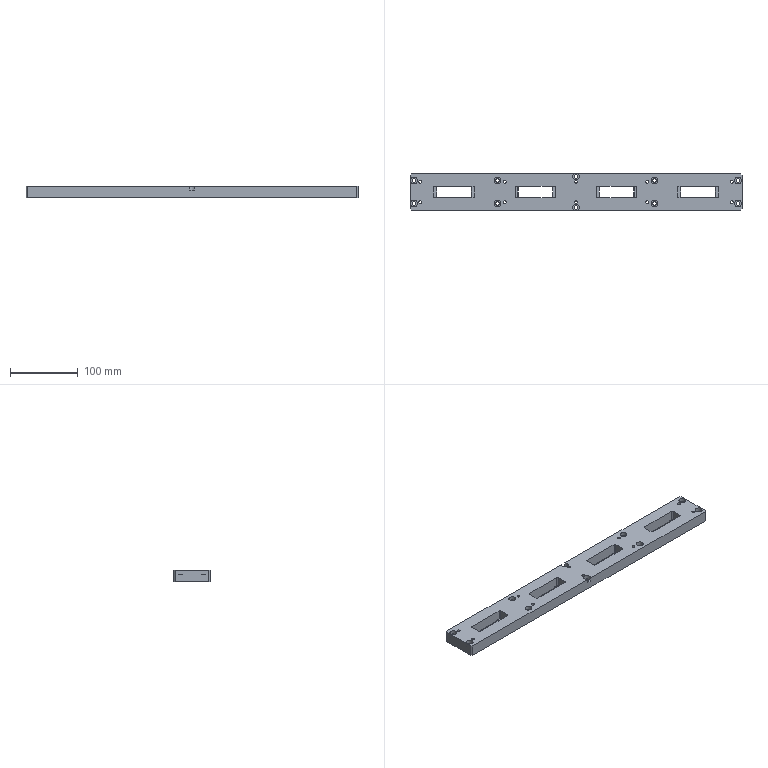NC program | NX | posted with a generic post | part box 490 x 54 x 17 mm
Lines 8259 to 8955 of 8955:
(ZLEVEL_PROFILE_2 , TOOL : D4R0.5)
N16468 T05 M6
N16470 G54
N16472 G17 G0 G90 X448.389 Y-32.658 S8500 M3
N16474 G43 Z30. H5
N16476 Z-13.1
N16478 G94 G1 Z-14.6 F2500.
N16480 X448.817 Y-33.4
N16482 G3 X449.164 Y-33.6 R0.4
N16484 G1 X449.175 Y-33.595
N16486 X449.187 Y-33.303
N16488 X449.191 Y-31.902
N16490 X449.189 Y-20.697
N16492 X449.179 Y-20.401
N16494 X449.164 Y-20.4
N16496 X449.093 Z-14.7
N16498 Y-33.6
N16500 X448.993 Z-14.8
N16502 Y-20.4
N16504 X448.893 Z-14.9
N16506 Y-33.6
N16508 X448.793 Z-15.
N16510 Y-20.4
N16512 X448.693 Z-15.1
N16514 Y-33.6
N16516 X448.575 Z-15.2
N16518 X448.588 Y-33.303
N16520 X448.591 Y-22.098
N16522 X448.579 Y-20.417
N16524 X448.577 Y-20.401
N16526 X448.552 Y-20.4
N16528 X448.163 Z-15.3
N16530 G2 X448.473 Y-20.487 R0.521
N16532 G1 X448.489 Y-22.098
N16534 X448.49 Y-32.182
N16536 X448.471 Y-33.537
N16538 X448.413 Y-33.562
N16540 X448.103 Y-33.6
N16542 X448.15 Y-33.54 Z-15.35
N16544 X448.198 Y-33.482 Z-15.4
N16546 X448.299 Y-33.481
N16548 X448.34 Y-33.48
N16550 X448.369 Y-33.451
N16552 X448.371 Y-33.41
N16554 X448.391 Y-31.622
N16556 Y-22.378
N16558 X448.372 Y-20.557
N16560 X448.367 Y-20.543
N16562 X448.189 Y-20.508
N16564 X448.265 Y-20.624 Z-15.5
N16566 X448.27 Y-20.625
N16568 X448.289 Y-22.098
N16570 X448.287 Y-31.902
N16572 X448.26 Y-33.369
N16574 Z-14.
N16576 G0 Z30.
N16578 X401.612 Y-21.343
N16580 Z-13.1
N16582 G1 Z-14.6
N16584 X401.183 Y-20.6
N16586 G3 X400.836 Y-20.4 R0.4
N16588 G1 X400.825 Y-20.405
N16590 X400.813 Y-20.697
N16592 X400.81 Y-21.818
N16594 X400.812 Y-33.303
N16596 X400.821 Y-33.599
N16598 X400.836 Y-33.6
N16600 X400.907 Z-14.7
N16602 Y-20.4
N16604 X401.007 Z-14.8
N16606 Y-33.6
N16608 X401.107 Z-14.9
N16610 Y-20.4
N16612 X401.207 Z-15.
N16614 Y-33.6
N16616 X401.307 Z-15.1
N16618 Y-20.4
N16620 Z-13.6
N16622 G0 X402.212 Y-21.243 Z-13.7
N16624 G1 Z-15.2
N16626 X401.841 Y-20.6
N16628 G3 X401.494 Y-20.4 R0.4
N16630 G1 X401.421 Y-20.417
N16632 X401.412 Y-20.697
N16634 X401.409 Y-31.902
N16636 X401.421 Y-33.583
N16638 X401.423 Y-33.599
N16640 X401.448 Y-33.6
N16642 X401.837 Z-15.3
N16644 G2 X401.528 Y-33.513 R0.52
N16646 G1 X401.511 Y-31.902
N16648 X401.51 Y-21.818
N16650 X401.53 Y-20.449
N16652 X401.587 Y-20.43
N16654 X401.857 Y-20.4
N16656 X401.848 Y-20.502 Z-15.4
N16658 G3 X401.641 Y-20.557 R0.405
N16660 G1 X401.629 Y-20.627
N16662 X401.607 Y-24.059
N16664 X401.609 Y-31.622
N16666 X401.628 Y-33.443
N16668 X401.633 Y-33.457
N16670 X401.811 Y-33.492
N16672 X401.736 Y-33.376 Z-15.5
N16674 X401.729 Y-33.373
N16676 X401.711 Y-31.902
N16678 X401.71 Y-22.378
N16680 X401.738 Y-20.625
N16682 Z-14.
N16684 G0 Z30.
N16686 X328.388 Y-32.657
N16688 Z-13.1
N16690 G1 Z-14.6
N16692 X328.817 Y-33.4
N16694 G3 X329.164 Y-33.6 R0.4
N16696 G1 X329.175 Y-33.595
N16698 X329.187 Y-33.303
N16700 X329.189 Y-32.182
N16702 Y-20.697
N16704 X329.179 Y-20.401
N16706 X329.164 Y-20.4
N16708 X329.093 Z-14.7
N16710 Y-33.6
N16712 X328.993 Z-14.8
N16714 Y-20.4
N16716 X328.893 Z-14.9
N16718 Y-33.6
N16720 X328.793 Z-15.
N16722 Y-20.4
N16724 X328.693 Z-15.1
N16726 Y-33.6
N16728 X328.575 Z-15.2
N16730 X328.588 Y-33.303
N16732 X328.591 Y-22.098
N16734 X328.579 Y-20.417
N16736 X328.577 Y-20.401
N16738 X328.552 Y-20.4
N16740 X328.163 Z-15.3
N16742 G2 X328.472 Y-20.487 R0.521
N16744 G1 X328.489 Y-22.098
N16746 X328.49 Y-32.182
N16748 X328.471 Y-33.537
N16750 X328.413 Y-33.562
N16752 X328.103 Y-33.6
N16754 X328.15 Y-33.54 Z-15.35
N16756 X328.198 Y-33.482 Z-15.4
N16758 X328.299 Y-33.481
N16760 X328.34 Y-33.48
N16762 X328.369 Y-33.451
N16764 X328.371 Y-33.41
N16766 X328.391 Y-31.622
N16768 Y-22.378
N16770 X328.372 Y-20.557
N16772 X328.367 Y-20.543
N16774 X328.189 Y-20.508
N16776 X328.265 Y-20.624 Z-15.5
N16778 X328.27 Y-20.625
N16780 X328.289 Y-22.098
N16782 X328.287 Y-31.902
N16784 X328.26 Y-33.369
N16786 Z-14.
N16788 G0 Z30.
N16790 X281.612 Y-21.343
N16792 Z-13.1
N16794 G1 Z-14.6
N16796 X281.183 Y-20.6
N16798 G3 X280.836 Y-20.4 R0.4
N16800 G1 X280.825 Y-20.405
N16802 X280.813 Y-20.697
N16804 X280.81 Y-21.818
N16806 X280.812 Y-33.303
N16808 X280.821 Y-33.599
N16810 X280.836 Y-33.6
N16812 X280.907 Z-14.7
N16814 Y-20.4
N16816 X281.007 Z-14.8
N16818 Y-33.6
N16820 X281.107 Z-14.9
N16822 Y-20.4
N16824 X281.207 Z-15.
N16826 Y-33.6
N16828 X281.307 Z-15.1
N16830 Y-20.4
N16832 Z-13.6
N16834 G0 X282.212 Y-21.243 Z-13.7
N16836 G1 Z-15.2
N16838 X281.841 Y-20.6
N16840 G3 X281.494 Y-20.4 R0.4
N16842 G1 X281.421 Y-20.417
N16844 X281.412 Y-20.697
N16846 X281.409 Y-31.902
N16848 X281.421 Y-33.583
N16850 X281.423 Y-33.599
N16852 X281.448 Y-33.6
N16854 X281.837 Z-15.3
N16856 G2 X281.528 Y-33.513 R0.52
N16858 G1 X281.511 Y-31.902
N16860 X281.51 Y-21.818
N16862 X281.53 Y-20.449
N16864 X281.587 Y-20.43
N16866 X281.857 Y-20.4
N16868 X281.848 Y-20.502 Z-15.4
N16870 G3 X281.641 Y-20.557 R0.405
N16872 G1 X281.629 Y-20.627
N16874 X281.607 Y-24.059
N16876 X281.609 Y-31.622
N16878 X281.628 Y-33.443
N16880 X281.633 Y-33.457
N16882 X281.811 Y-33.492
N16884 X281.736 Y-33.376 Z-15.5
N16886 X281.729 Y-33.373
N16888 X281.711 Y-31.902
N16890 X281.71 Y-22.378
N16892 X281.738 Y-20.625
N16894 Z-14.
N16896 G0 Z30.
N16898 X208.389 Y-32.658
N16900 Z-13.1
N16902 G1 Z-14.6
N16904 X208.817 Y-33.4
N16906 G3 X209.164 Y-33.6 R0.4
N16908 G1 X209.175 Y-33.595
N16910 X209.187 Y-33.303
N16912 X209.191 Y-31.902
N16914 X209.189 Y-20.697
N16916 X209.179 Y-20.401
N16918 X209.164 Y-20.4
N16920 X209.093 Z-14.7
N16922 Y-33.6
N16924 X208.993 Z-14.8
N16926 Y-20.4
N16928 X208.893 Z-14.9
N16930 Y-33.6
N16932 X208.793 Z-15.
N16934 Y-20.4
N16936 X208.693 Z-15.1
N16938 Y-33.6
N16940 X208.575 Z-15.2
N16942 X208.588 Y-33.303
N16944 X208.591 Y-22.098
N16946 X208.579 Y-20.417
N16948 X208.577 Y-20.401
N16950 X208.552 Y-20.4
N16952 X208.163 Z-15.3
N16954 G2 X208.472 Y-20.487 R0.521
N16956 G1 X208.489 Y-22.098
N16958 X208.49 Y-32.182
N16960 X208.471 Y-33.537
N16962 X208.413 Y-33.562
N16964 X208.103 Y-33.6
N16966 X208.15 Y-33.54 Z-15.35
N16968 X208.198 Y-33.482 Z-15.4
N16970 X208.299 Y-33.481
N16972 X208.34 Y-33.48
N16974 X208.369 Y-33.451
N16976 X208.371 Y-33.41
N16978 X208.391 Y-31.622
N16980 Y-22.378
N16982 X208.372 Y-20.557
N16984 X208.367 Y-20.543
N16986 X208.189 Y-20.508
N16988 X208.265 Y-20.624 Z-15.5
N16990 X208.27 Y-20.625
N16992 X208.289 Y-22.098
N16994 X208.287 Y-31.902
N16996 X208.26 Y-33.369
N16998 Z-14.
N17000 G0 Z30.
N17002 X161.612 Y-21.343
N17004 Z-13.1
N17006 G1 Z-14.6
N17008 X161.183 Y-20.6
N17010 G3 X160.836 Y-20.4 R0.4
N17012 G1 X160.825 Y-20.405
N17014 X160.813 Y-20.697
N17016 X160.81 Y-21.818
N17018 X160.812 Y-33.303
N17020 X160.821 Y-33.599
N17022 X160.836 Y-33.6
N17024 X160.907 Z-14.7
N17026 Y-20.4
N17028 X161.007 Z-14.8
N17030 Y-33.6
N17032 X161.107 Z-14.9
N17034 Y-20.4
N17036 X161.207 Z-15.
N17038 Y-33.6
N17040 X161.307 Z-15.1
N17042 Y-20.4
N17044 Z-13.6
N17046 G0 X162.212 Y-21.243 Z-13.7
N17048 G1 Z-15.2
N17050 X161.841 Y-20.6
N17052 G3 X161.494 Y-20.4 R0.4
N17054 G1 X161.421 Y-20.417
N17056 X161.412 Y-20.697
N17058 X161.409 Y-31.902
N17060 X161.421 Y-33.583
N17062 X161.423 Y-33.599
N17064 X161.448 Y-33.6
N17066 X161.837 Z-15.3
N17068 G2 X161.528 Y-33.513 R0.52
N17070 G1 X161.511 Y-31.902
N17072 X161.51 Y-21.818
N17074 X161.53 Y-20.449
N17076 X161.587 Y-20.43
N17078 X161.857 Y-20.4
N17080 X161.848 Y-20.502 Z-15.4
N17082 G3 X161.641 Y-20.557 R0.405
N17084 G1 X161.629 Y-20.627
N17086 X161.607 Y-24.059
N17088 X161.609 Y-31.622
N17090 X161.628 Y-33.443
N17092 X161.633 Y-33.457
N17094 X161.811 Y-33.492
N17096 X161.736 Y-33.376 Z-15.5
N17098 X161.729 Y-33.373
N17100 X161.711 Y-31.902
N17102 X161.71 Y-22.378
N17104 X161.738 Y-20.625
N17106 Z-14.
N17108 G0 Z30.
N17110 X88.389 Y-32.658
N17112 Z-13.1
N17114 G1 Z-14.6
N17116 X88.817 Y-33.4
N17118 G3 X89.164 Y-33.6 R0.4
N17120 G1 X89.175 Y-33.595
N17122 X89.187 Y-33.303
N17124 X89.191 Y-31.902
N17126 X89.189 Y-20.697
N17128 X89.179 Y-20.401
N17130 X89.164 Y-20.4
N17132 X89.093 Z-14.7
N17134 Y-33.6
N17136 X88.993 Z-14.8
N17138 Y-20.4
N17140 X88.893 Z-14.9
N17142 Y-33.6
N17144 X88.793 Z-15.
N17146 Y-20.4
N17148 X88.693 Z-15.1
N17150 Y-33.6
N17152 X88.575 Z-15.2
N17154 X88.588 Y-33.303
N17156 X88.591 Y-22.098
N17158 X88.579 Y-20.417
N17160 X88.577 Y-20.401
N17162 X88.552 Y-20.4
N17164 X88.163 Z-15.3
N17166 G2 X88.472 Y-20.487 R0.521
N17168 G1 X88.489 Y-22.098
N17170 X88.49 Y-32.182
N17172 X88.471 Y-33.537
N17174 X88.413 Y-33.562
N17176 X88.103 Y-33.6
N17178 X88.15 Y-33.54 Z-15.35
N17180 X88.198 Y-33.482 Z-15.4
N17182 X88.299 Y-33.481
N17184 X88.34 Y-33.48
N17186 X88.369 Y-33.451
N17188 X88.371 Y-33.41
N17190 X88.391 Y-31.622
N17192 Y-22.378
N17194 X88.372 Y-20.557
N17196 X88.367 Y-20.543
N17198 X88.189 Y-20.508
N17200 X88.265 Y-20.624 Z-15.5
N17202 X88.27 Y-20.625
N17204 X88.289 Y-22.098
N17206 X88.287 Y-31.902
N17208 X88.26 Y-33.369
N17210 Z-14.
N17212 G0 Z30.
N17214 X41.612 Y-21.343
N17216 Z-13.1
N17218 G1 Z-14.6
N17220 X41.183 Y-20.6
N17222 G3 X40.836 Y-20.4 R0.4
N17224 G1 X40.825 Y-20.405
N17226 X40.813 Y-20.697
N17228 X40.81 Y-21.818
N17230 X40.812 Y-33.303
N17232 X40.821 Y-33.599
N17234 X40.836 Y-33.6
N17236 X40.907 Z-14.7
N17238 Y-20.4
N17240 X41.007 Z-14.8
N17242 Y-33.6
N17244 X41.107 Z-14.9
N17246 Y-20.4
N17248 X41.207 Z-15.
N17250 Y-33.6
N17252 X41.307 Z-15.1
N17254 Y-20.4
N17256 Z-13.6
N17258 G0 X42.212 Y-21.243 Z-13.7
N17260 G1 Z-15.2
N17262 X41.841 Y-20.6
N17264 G3 X41.494 Y-20.4 R0.4
N17266 G1 X41.421 Y-20.417
N17268 X41.412 Y-20.697
N17270 X41.409 Y-31.902
N17272 X41.421 Y-33.583
N17274 X41.423 Y-33.599
N17276 X41.448 Y-33.6
N17278 X41.837 Z-15.3
N17280 G2 X41.528 Y-33.513 R0.52
N17282 G1 X41.511 Y-31.902
N17284 X41.51 Y-21.818
N17286 X41.53 Y-20.449
N17288 X41.587 Y-20.43
N17290 X41.857 Y-20.4
N17292 X41.848 Y-20.502 Z-15.4
N17294 G3 X41.641 Y-20.557 R0.405
N17296 G1 X41.629 Y-20.627
N17298 X41.607 Y-24.059
N17300 X41.609 Y-31.622
N17302 X41.628 Y-33.443
N17304 X41.633 Y-33.457
N17306 X41.811 Y-33.492
N17308 X41.736 Y-33.376 Z-15.5
N17310 X41.729 Y-33.373
N17312 X41.711 Y-31.902
N17314 X41.71 Y-22.378
N17316 X41.738 Y-20.625
N17318 Z-14.
N17320 G0 Z30.
N17322 M5
(PLANAR_MILL_COPY , TOOL : D6A45)
N17324 T01 M6
N17326 G54
N17328 G17 G0 G90 X2.4 Y-43.134 S8500 M3
N17330 G43 Z30. H1
N17332 Z0.5
N17334 G94 G1 Z-1. F1250.
N17336 G3 X1.9 Y-44. R1.
N17338 X6. Y-48.1 R4.1
N17340 X1.9 Y-44. R-4.1
N17342 X2.4 Y-44.866 R1.
N17344 G1 Z0.5
N17346 G0 Z30.
N17348 X14.134 Y-42.7
N17350 Z0.5
N17352 G1 Z-1.
N17354 G3 X15. Y-43.2 R1.
N17356 X16.2 Y-42. R1.2
N17358 X15. Y-43.2 R-1.2
N17360 X15.866 Y-42.7 R1.
N17362 G1 Z0.5
N17364 G0 Z30.
N17366 X2.4 Y-9.134
N17368 Z0.5
N17370 G1 Z-1.
N17372 G3 X1.9 Y-10. R1.
N17374 X6. Y-14.1 R4.1
N17376 X1.9 Y-10. R-4.1
N17378 X2.4 Y-10.866 R1.
N17380 G1 Z0.5
N17382 G0 Z30.
N17384 X15.866 Y-11.3
N17386 Z0.5
N17388 G1 Z-1.
N17390 G3 X15. Y-10.8 R1.
N17392 X13.8 Y-12. R1.2
N17394 X15. Y-10.8 R-1.2
N17396 X14.134 Y-11.3 R1.
N17398 G1 Z0.5
N17400 G0 Z30.
N17402 X65.866 Y-19.8
N17404 Z0.5
N17406 G1 Z-1.
N17408 G3 X65. Y-19.3 R1.
N17410 G1 X37.
N17412 G3 X35.9 Y-20.4 R1.1
N17414 G1 Y-33.6
N17416 G3 X37. Y-34.7 R1.1
N17418 G1 X93.
N17420 G3 X94.1 Y-33.6 R1.1
N17422 G1 Y-20.4
N17424 G3 X93. Y-19.3 R1.1
N17426 G1 X65.
N17428 G3 X64.134 Y-19.8 R1.
N17430 G1 Z0.5
N17432 G0 Z30.
N17434 X129.866 Y-6.4
N17436 Z0.5
N17438 G1 Z-1.
N17440 G3 X129. Y-5.9 R1.
N17442 X124.9 Y-10. R4.1
N17444 X129. Y-5.9 R-4.1
N17446 X128.134 Y-6.4 R1.
N17448 G1 Z0.5
N17450 G0 Z30.
N17452 X140.866 Y-11.3
N17454 Z0.5
N17456 G1 Z-1.
N17458 G3 X140. Y-10.8 R1.
N17460 X138.8 Y-12. R1.2
N17462 X140. Y-10.8 R-1.2
N17464 X139.134 Y-11.3 R1.
N17466 G1 Z0.5
N17468 G0 Z30.
N17470 X128.134 Y-47.6
N17472 Z0.5
N17474 G1 Z-1.
N17476 G3 X129. Y-48.1 R1.
N17478 X133.1 Y-44. R4.1
N17480 X129. Y-48.1 R-4.1
N17482 X129.866 Y-47.6 R1.
N17484 G1 Z0.5
N17486 G0 Z30.
N17488 X139.134 Y-42.7
N17490 Z0.5
N17492 G1 Z-1.
N17494 G3 X140. Y-43.2 R1.
N17496 X141.2 Y-42. R1.2
N17498 X140. Y-43.2 R-1.2
N17500 X140.866 Y-42.7 R1.
N17502 G1 Z0.5
N17504 G0 Z30.
N17506 X184.134 Y-34.2
N17508 Z0.5
N17510 G1 Z-1.
N17512 G3 X185. Y-34.7 R1.
N17514 G1 X213.
N17516 G3 X214.1 Y-33.6 R1.1
N17518 G1 Y-20.4
N17520 G3 X213. Y-19.3 R1.1
N17522 G1 X157.
N17524 G3 X155.9 Y-20.4 R1.1
N17526 G1 Y-33.6
N17528 G3 X157. Y-34.7 R1.1
N17530 G1 X185.
N17532 G3 X185.866 Y-34.2 R1.
N17534 G1 Z0.5
N17536 G0 Z30.
N17538 X245.866 Y-11.3
N17540 Z0.5
N17542 G1 Z-1.
N17544 G3 X245. Y-10.8 R1.
N17546 X243.8 Y-12. R1.2
N17548 X245. Y-10.8 R-1.2
N17550 X244.134 Y-11.3 R1.
N17552 G1 Z0.5
N17554 G0 Z30.
N17556 X121.134 Y1.4
N17558 Z0.5
N17560 G1 Z-1.
N17562 G3 X122. Y0.9 R1.
N17564 G1 X242.
N17566 G2 X242.54 Y-0.72 R0.9
N17568 G3 X247.46 Y-0.72 R-4.1
N17570 G2 X248. Y0.9 R0.9
N17572 G1 X488.
N17574 G2 X488.636 Y0.636 R0.9
N17576 G1 X490.636 Y-1.364
N17578 G2 X490.9 Y-2. R0.9
N17580 G1 Y-52.
N17582 G2 X490.636 Y-52.636 R0.9
N17584 G1 X488.636 Y-54.636
N17586 G2 X488. Y-54.9 R0.9
N17588 G1 X248.
N17590 G2 X247.46 Y-53.28 R0.9
N17592 G3 X242.54 Y-53.28 R-4.1
N17594 G2 X242. Y-54.9 R0.9
N17596 G1 X2.
N17598 G2 X1.364 Y-54.636 R0.9
N17600 G1 X-0.636 Y-52.636
N17602 G2 X-0.9 Y-52. R0.9
N17604 G1 Y-2.
N17606 G2 X-0.636 Y-1.364 R0.9
N17608 G1 X1.364 Y0.636
N17610 G2 X2. Y0.9 R0.9
N17612 G1 X122.
N17614 G3 X122.866 Y1.4 R1.
N17616 G1 Z0.5
N17618 G0 Z30.
N17620 X244.134 Y-42.7
N17622 Z0.5
N17624 G1 Z-1.
N17626 G3 X245. Y-43.2 R1.
N17628 X246.2 Y-42. R1.2
N17630 X245. Y-43.2 R-1.2
N17632 X245.866 Y-42.7 R1.
N17634 G1 Z0.5
N17636 G0 Z30.
N17638 X304.134 Y-34.2
N17640 Z0.5
N17642 G1 Z-1.
N17644 G3 X305. Y-34.7 R1.
N17646 G1 X333.
N17648 G3 X334.1 Y-33.6 R1.1
N17650 G1 Y-20.4
N17652 G3 X333. Y-19.3 R1.1
N17654 G1 X277.
N17656 G3 X275.9 Y-20.4 R1.1
N17658 G1 Y-33.6
N17660 G3 X277. Y-34.7 R1.1
N17662 G1 X305.
N17664 G3 X305.866 Y-34.2 R1.
N17666 G1 Z0.5
N17668 G0 Z30.
N17670 X349.134 Y-42.7
N17672 Z0.5
N17674 G1 Z-1.
N17676 G3 X350. Y-43.2 R1.
N17678 X351.2 Y-42. R1.2
N17680 X350. Y-43.2 R-1.2
N17682 X350.866 Y-42.7 R1.
N17684 G1 Z0.5
N17686 G0 Z30.
N17688 X360.134 Y-47.6
N17690 Z0.5
N17692 G1 Z-1.
N17694 G3 X361. Y-48.1 R1.
N17696 X365.1 Y-44. R4.1
N17698 X361. Y-48.1 R-4.1
N17700 X361.866 Y-47.6 R1.
N17702 G1 Z0.5
N17704 G0 Z30.
N17706 X350.866 Y-11.3
N17708 Z0.5
N17710 G1 Z-1.
N17712 G3 X350. Y-10.8 R1.
N17714 X348.8 Y-12. R1.2
N17716 X350. Y-10.8 R-1.2
N17718 X349.134 Y-11.3 R1.
N17720 G1 Z0.5
N17722 G0 Z30.
N17724 X361.866 Y-6.4
N17726 Z0.5
N17728 G1 Z-1.
N17730 G3 X361. Y-5.9 R1.
N17732 X356.9 Y-10. R4.1
N17734 X361. Y-5.9 R-4.1
N17736 X360.134 Y-6.4 R1.
N17738 G1 Z0.5
N17740 G0 Z30.
N17742 X425.866 Y-19.8
N17744 Z0.5
N17746 G1 Z-1.
N17748 G3 X425. Y-19.3 R1.
N17750 G1 X397.
N17752 G3 X395.9 Y-20.4 R1.1
N17754 G1 Y-33.6
N17756 G3 X397. Y-34.7 R1.1
N17758 G1 X453.
N17760 G3 X454.1 Y-33.6 R1.1
N17762 G1 Y-20.4
N17764 G3 X453. Y-19.3 R1.1
N17766 G1 X425.
N17768 G3 X424.134 Y-19.8 R1.
N17770 G1 Z0.5
N17772 G0 Z30.
N17774 X475.866 Y-11.3
N17776 Z0.5
N17778 G1 Z-1.
N17780 G3 X475. Y-10.8 R1.
N17782 X473.8 Y-12. R1.2
N17784 X475. Y-10.8 R-1.2
N17786 X474.134 Y-11.3 R1.
N17788 G1 Z0.5
N17790 G0 Z30.
N17792 X487.6 Y-10.866
N17794 Z0.5
N17796 G1 Z-1.
N17798 G3 X488.1 Y-10. R1.
N17800 X484. Y-5.9 R4.1
N17802 X488.1 Y-10. R-4.1
N17804 X487.6 Y-9.134 R1.
N17806 G1 Z0.5
N17808 G0 Z30.
N17810 X474.134 Y-42.7
N17812 Z0.5
N17814 G1 Z-1.
N17816 G3 X475. Y-43.2 R1.
N17818 X476.2 Y-42. R1.2
N17820 X475. Y-43.2 R-1.2
N17822 X475.866 Y-42.7 R1.
N17824 G1 Z0.5
N17826 G0 Z30.
N17828 X487.6 Y-44.866
N17830 Z0.5
N17832 G1 Z-1.
N17834 G3 X488.1 Y-44. R1.
N17836 X484. Y-39.9 R4.1
N17838 X488.1 Y-44. R-4.1
N17840 X487.6 Y-43.134 R1.
N17842 G1 Z0.5
N17844 G0 Z30.
N17846 M5
N17848 M2